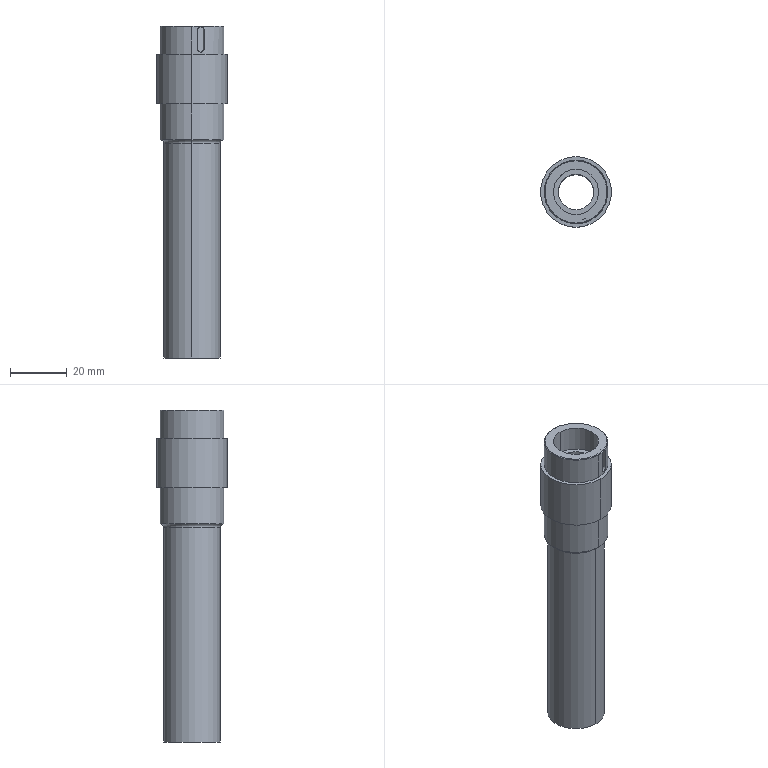Part | STEP file | 2026.6.15-Main Assembly图.sldasm-Part-95 | 1 solid | 26 faces | box 25 x 25 x 117.405 mm | volume 26751 mm3 | cylinder 14 | plane 8 | cone 2 | torus 2 | commonest cylinder face diameters 22.5 x4 2.5 x2 12.5 x2 16 x2 20 x2 25 x2
STEP:
#1=CARTESIAN_POINT('',(-1571.233,1430.514,3525.142));
#2=VERTEX_POINT('',#1);
#3=CARTESIAN_POINT('',(-1571.243,1418.014,3525.142));
#4=VERTEX_POINT('',#3);
#5=CARTESIAN_POINT('',(-1571.238,1424.264,3525.142));
#6=DIRECTION('',(0.,0.,1.));
#7=DIRECTION('',(1.,0.,0.));
#8=AXIS2_PLACEMENT_3D('',#5,#6,#7);
#9=CIRCLE('',#8,6.25);
#10=EDGE_CURVE('',#2,#4,#9,.T.);
#11=ORIENTED_EDGE('',*,*,#10,.F.);
#12=CARTESIAN_POINT('',(-1571.233,1430.514,3633.547));
#13=VERTEX_POINT('',#12);
#14=CARTESIAN_POINT('',(-1571.233,1430.514,3314.147));
#15=DIRECTION('',(0.,0.,1.));
#16=VECTOR('',#15,1000.);
#17=LINE('',#14,#16);
#18=EDGE_CURVE('',#2,#13,#17,.T.);
#19=ORIENTED_EDGE('',*,*,#18,.T.);
#20=CARTESIAN_POINT('',(-1571.243,1418.014,3633.547));
#21=VERTEX_POINT('',#20);
#22=CARTESIAN_POINT('',(-1571.238,1424.264,3633.547));
#23=DIRECTION('',(0.,0.,1.));
#24=DIRECTION('',(-0.0007664,-1.,0.));
#25=AXIS2_PLACEMENT_3D('',#22,#23,#24);
#26=CIRCLE('',#25,6.25);
#27=EDGE_CURVE('',#13,#21,#26,.T.);
#28=ORIENTED_EDGE('',*,*,#27,.T.);
#29=CARTESIAN_POINT('',(-1571.243,1418.014,3314.147));
#30=DIRECTION('',(0.,0.,1.));
#31=VECTOR('',#30,1000.);
#32=LINE('',#29,#31);
#33=EDGE_CURVE('',#4,#21,#32,.T.);
#34=ORIENTED_EDGE('',*,*,#33,.F.);
#35=EDGE_LOOP('',(#11,#19,#28,#34));
#36=FACE_OUTER_BOUND('',#35,.T.);
#37=CARTESIAN_POINT('',(-1571.238,1424.264,3314.147));
#38=DIRECTION('',(0.,0.,1.));
#39=DIRECTION('',(-0.0007664,-1.,0.));
#40=AXIS2_PLACEMENT_3D('',#37,#38,#39);
#41=CYLINDRICAL_SURFACE('',#40,6.25);
#42=ADVANCED_FACE('',(#36),#41,.F.);
#43=CARTESIAN_POINT('',(-1571.232,1432.264,3633.547));
#44=VERTEX_POINT('',#43);
#45=CARTESIAN_POINT('',(-1571.244,1416.264,3633.547));
#46=VERTEX_POINT('',#45);
#47=CARTESIAN_POINT('',(-1571.238,1424.264,3633.547));
#48=DIRECTION('',(0.,0.,1.));
#49=DIRECTION('',(-0.0007664,-1.,0.));
#50=AXIS2_PLACEMENT_3D('',#47,#48,#49);
#51=CIRCLE('',#50,8.);
#52=EDGE_CURVE('',#44,#46,#51,.T.);
#53=ORIENTED_EDGE('',*,*,#52,.F.);
#54=CARTESIAN_POINT('',(-1571.232,1432.264,3642.547));
#55=VERTEX_POINT('',#54);
#56=CARTESIAN_POINT('',(-1571.232,1432.264,3314.147));
#57=DIRECTION('',(0.,0.,1.));
#58=VECTOR('',#57,1000.);
#59=LINE('',#56,#58);
#60=EDGE_CURVE('',#44,#55,#59,.T.);
#61=ORIENTED_EDGE('',*,*,#60,.T.);
#62=CARTESIAN_POINT('',(-1571.244,1416.264,3642.547));
#63=VERTEX_POINT('',#62);
#64=CARTESIAN_POINT('',(-1571.238,1424.264,3642.547));
#65=DIRECTION('',(0.,0.,1.));
#66=DIRECTION('',(-0.0007664,-1.,0.));
#67=AXIS2_PLACEMENT_3D('',#64,#65,#66);
#68=CIRCLE('',#67,8.);
#69=EDGE_CURVE('',#55,#63,#68,.T.);
#70=ORIENTED_EDGE('',*,*,#69,.T.);
#71=CARTESIAN_POINT('',(-1571.244,1416.264,3314.147));
#72=DIRECTION('',(0.,0.,1.));
#73=VECTOR('',#72,1000.);
#74=LINE('',#71,#73);
#75=EDGE_CURVE('',#46,#63,#74,.T.);
#76=ORIENTED_EDGE('',*,*,#75,.F.);
#77=EDGE_LOOP('',(#53,#61,#70,#76));
#78=FACE_OUTER_BOUND('',#77,.T.);
#79=CARTESIAN_POINT('',(-1571.238,1424.264,3314.147));
#80=DIRECTION('',(0.,0.,1.));
#81=DIRECTION('',(-0.0007664,-1.,0.));
#82=AXIS2_PLACEMENT_3D('',#79,#80,#81);
#83=CYLINDRICAL_SURFACE('',#82,8.);
#84=ADVANCED_FACE('',(#78),#83,.F.);
#85=CARTESIAN_POINT('',(-1571.247,1413.264,3642.547));
#86=VERTEX_POINT('',#85);
#87=CARTESIAN_POINT('',(-1571.23,1435.264,3642.547));
#88=VERTEX_POINT('',#87);
#89=CARTESIAN_POINT('',(-1571.238,1424.264,3642.547));
#90=DIRECTION('',(0.,0.,1.));
#91=DIRECTION('',(-0.0007664,-1.,0.));
#92=AXIS2_PLACEMENT_3D('',#89,#90,#91);
#93=CIRCLE('',#92,11.);
#94=EDGE_CURVE('',#86,#88,#93,.T.);
#95=ORIENTED_EDGE('',*,*,#94,.F.);
#96=CARTESIAN_POINT('',(-1571.247,1413.014,3642.297));
#97=VERTEX_POINT('',#96);
#98=CARTESIAN_POINT('',(-1571.247,1413.264,3642.547));
#99=DIRECTION('',(-0.000542,-0.7071,-0.7071));
#100=VECTOR('',#99,1000.);
#101=LINE('',#98,#100);
#102=EDGE_CURVE('',#86,#97,#101,.T.);
#103=ORIENTED_EDGE('',*,*,#102,.T.);
#104=CARTESIAN_POINT('',(-1568.056,1413.474,3642.297));
#105=VERTEX_POINT('',#104);
#106=CARTESIAN_POINT('',(-1571.238,1424.264,3642.297));
#107=DIRECTION('',(0.,0.,1.));
#108=DIRECTION('',(-0.0007664,-1.,0.));
#109=AXIS2_PLACEMENT_3D('',#106,#107,#108);
#110=CIRCLE('',#109,11.25);
#111=EDGE_CURVE('',#97,#105,#110,.T.);
#112=ORIENTED_EDGE('',*,*,#111,.T.);
#113=CARTESIAN_POINT('',(-1571.23,1435.514,3642.297));
#114=VERTEX_POINT('',#113);
#115=CARTESIAN_POINT('',(-1571.238,1424.264,3642.297));
#116=DIRECTION('',(0.,0.,1.));
#117=DIRECTION('',(-0.0007664,-1.,0.));
#118=AXIS2_PLACEMENT_3D('',#115,#116,#117);
#119=CIRCLE('',#118,11.25);
#120=EDGE_CURVE('',#105,#114,#119,.T.);
#121=ORIENTED_EDGE('',*,*,#120,.T.);
#122=CARTESIAN_POINT('',(-1571.23,1435.264,3642.547));
#123=DIRECTION('',(0.000542,0.7071,-0.7071));
#124=VECTOR('',#123,1000.);
#125=LINE('',#122,#124);
#126=EDGE_CURVE('',#88,#114,#125,.T.);
#127=ORIENTED_EDGE('',*,*,#126,.F.);
#128=EDGE_LOOP('',(#95,#103,#112,#121,#127));
#129=FACE_OUTER_BOUND('',#128,.T.);
#130=CARTESIAN_POINT('',(-1571.238,1424.264,3642.547));
#131=DIRECTION('',(0.,0.,-1.));
#132=DIRECTION('',(0.0007664,1.,0.));
#133=AXIS2_PLACEMENT_3D('',#130,#131,#132);
#134=CONICAL_SURFACE('',#133,11.,0.7854);
#135=ADVANCED_FACE('',(#129),#134,.T.);
#136=CARTESIAN_POINT('',(-1571.247,1413.014,3632.547));
#137=VERTEX_POINT('',#136);
#138=CARTESIAN_POINT('',(-1571.23,1435.514,3632.547));
#139=VERTEX_POINT('',#138);
#140=CARTESIAN_POINT('',(-1571.238,1424.264,3632.547));
#141=DIRECTION('',(0.,0.,1.));
#142=DIRECTION('',(-0.0007664,-1.,0.));
#143=AXIS2_PLACEMENT_3D('',#140,#141,#142);
#144=CIRCLE('',#143,11.25);
#145=EDGE_CURVE('',#137,#139,#144,.T.);
#146=ORIENTED_EDGE('',*,*,#145,.T.);
#147=CARTESIAN_POINT('',(-1571.23,1435.514,3314.147));
#148=DIRECTION('',(0.,0.,1.));
#149=VECTOR('',#148,1000.);
#150=LINE('',#147,#149);
#151=EDGE_CURVE('',#139,#114,#150,.T.);
#152=ORIENTED_EDGE('',*,*,#151,.T.);
#153=ORIENTED_EDGE('',*,*,#120,.F.);
#154=CARTESIAN_POINT('',(-1566.877,1413.894,3641.047));
#155=VERTEX_POINT('',#154);
#156=CARTESIAN_POINT('',(-1566.877,1413.894,3641.047));
#157=CARTESIAN_POINT('',(-1566.877,1413.894,3641.212));
#158=CARTESIAN_POINT('',(-1566.907,1413.881,3641.374));
#159=CARTESIAN_POINT('',(-1567.024,1413.833,3641.677));
#160=CARTESIAN_POINT('',(-1567.11,1413.798,3641.816));
#161=CARTESIAN_POINT('',(-1567.326,1413.716,3642.046));
#162=CARTESIAN_POINT('',(-1567.458,1413.668,3642.139));
#163=CARTESIAN_POINT('',(-1567.743,1413.57,3642.264));
#164=CARTESIAN_POINT('',(-1567.899,1413.52,3642.297));
#165=CARTESIAN_POINT('',(-1568.056,1413.474,3642.297));
#166=B_SPLINE_CURVE_WITH_KNOTS('',3,(#156,#157,#158,#159,#160,#161,#162,#163,#164,#165),.UNSPECIFIED.,.F.,.F.,(4,2,2,2,4),(0.,0.000489,0.000978,0.001467,0.001956),.UNSPECIFIED.);
#167=EDGE_CURVE('',#155,#105,#166,.T.);
#168=ORIENTED_EDGE('',*,*,#167,.F.);
#169=CARTESIAN_POINT('',(-1566.877,1413.894,3634.547));
#170=VERTEX_POINT('',#169);
#171=CARTESIAN_POINT('',(-1566.877,1413.894,3314.147));
#172=DIRECTION('',(0.,0.,-1.));
#173=VECTOR('',#172,1000.);
#174=LINE('',#171,#173);
#175=EDGE_CURVE('',#155,#170,#174,.T.);
#176=ORIENTED_EDGE('',*,*,#175,.T.);
#177=CARTESIAN_POINT('',(-1569.275,1413.187,3634.547));
#178=VERTEX_POINT('',#177);
#179=CARTESIAN_POINT('',(-1569.275,1413.187,3634.547));
#180=CARTESIAN_POINT('',(-1569.275,1413.187,3634.382));
#181=CARTESIAN_POINT('',(-1569.242,1413.193,3634.219));
#182=CARTESIAN_POINT('',(-1569.118,1413.216,3633.917));
#183=CARTESIAN_POINT('',(-1569.027,1413.233,3633.778));
#184=CARTESIAN_POINT('',(-1568.801,1413.281,3633.548));
#185=CARTESIAN_POINT('',(-1568.664,1413.312,3633.455));
#186=CARTESIAN_POINT('',(-1568.372,1413.384,3633.33));
#187=CARTESIAN_POINT('',(-1568.213,1413.427,3633.297));
#188=CARTESIAN_POINT('',(-1567.979,1413.497,3633.297));
#189=CARTESIAN_POINT('',(-1567.899,1413.521,3633.305));
#190=CARTESIAN_POINT('',(-1567.747,1413.57,3633.337));
#191=CARTESIAN_POINT('',(-1567.673,1413.594,3633.36));
#192=CARTESIAN_POINT('',(-1567.457,1413.668,3633.454));
#193=CARTESIAN_POINT('',(-1567.328,1413.715,3633.546));
#194=CARTESIAN_POINT('',(-1567.109,1413.799,3633.779));
#195=CARTESIAN_POINT('',(-1567.024,1413.833,3633.916));
#196=CARTESIAN_POINT('',(-1566.907,1413.881,3634.219));
#197=CARTESIAN_POINT('',(-1566.877,1413.894,3634.382));
#198=CARTESIAN_POINT('',(-1566.877,1413.894,3634.547));
#199=B_SPLINE_CURVE_WITH_KNOTS('',3,(#179,#180,#181,#182,#183,#184,#185,#186,#187,#188,#189,#190,#191,#192,#193,#194,#195,#196,#197,#198),.UNSPECIFIED.,.F.,.F.,(4,2,2,2,2,2,2,2,2,4),(0.,0.0004888,0.0009776,0.001466,0.001955,0.002199,0.002444,0.002933,0.003421,0.00391),.UNSPECIFIED.);
#200=EDGE_CURVE('',#178,#170,#199,.T.);
#201=ORIENTED_EDGE('',*,*,#200,.F.);
#202=CARTESIAN_POINT('',(-1569.275,1413.187,3641.047));
#203=VERTEX_POINT('',#202);
#204=CARTESIAN_POINT('',(-1569.275,1413.187,3314.147));
#205=DIRECTION('',(0.,0.,1.));
#206=VECTOR('',#205,1000.);
#207=LINE('',#204,#206);
#208=EDGE_CURVE('',#178,#203,#207,.T.);
#209=ORIENTED_EDGE('',*,*,#208,.T.);
#210=CARTESIAN_POINT('',(-1568.056,1413.474,3642.297));
#211=CARTESIAN_POINT('',(-1568.134,1413.451,3642.297));
#212=CARTESIAN_POINT('',(-1568.214,1413.428,3642.289));
#213=CARTESIAN_POINT('',(-1568.369,1413.386,3642.257));
#214=CARTESIAN_POINT('',(-1568.444,1413.367,3642.233));
#215=CARTESIAN_POINT('',(-1568.665,1413.312,3642.139));
#216=CARTESIAN_POINT('',(-1568.799,1413.281,3642.048));
#217=CARTESIAN_POINT('',(-1569.028,1413.233,3641.814));
#218=CARTESIAN_POINT('',(-1569.118,1413.216,3641.677));
#219=CARTESIAN_POINT('',(-1569.242,1413.193,3641.375));
#220=CARTESIAN_POINT('',(-1569.275,1413.187,3641.212));
#221=CARTESIAN_POINT('',(-1569.275,1413.187,3641.047));
#222=B_SPLINE_CURVE_WITH_KNOTS('',3,(#210,#211,#212,#213,#214,#215,#216,#217,#218,#219,#220,#221),.UNSPECIFIED.,.F.,.F.,(4,2,2,2,2,4),(0.001956,0.0022,0.002445,0.002933,0.003422,0.00391),.UNSPECIFIED.);
#223=EDGE_CURVE('',#105,#203,#222,.T.);
#224=ORIENTED_EDGE('',*,*,#223,.F.);
#225=ORIENTED_EDGE('',*,*,#111,.F.);
#226=CARTESIAN_POINT('',(-1571.247,1413.014,3314.147));
#227=DIRECTION('',(0.,0.,1.));
#228=VECTOR('',#227,1000.);
#229=LINE('',#226,#228);
#230=EDGE_CURVE('',#137,#97,#229,.T.);
#231=ORIENTED_EDGE('',*,*,#230,.F.);
#232=EDGE_LOOP('',(#146,#152,#153,#168,#176,#201,#209,#224,#225,#231));
#233=FACE_OUTER_BOUND('',#232,.T.);
#234=CARTESIAN_POINT('',(-1571.238,1424.264,3314.147));
#235=DIRECTION('',(0.,0.,1.));
#236=DIRECTION('',(-0.0007664,-1.,0.));
#237=AXIS2_PLACEMENT_3D('',#234,#235,#236);
#238=CYLINDRICAL_SURFACE('',#237,11.25);
#239=ADVANCED_FACE('',(#233),#238,.T.);
#240=CARTESIAN_POINT('',(-1571.231,1434.264,3525.142));
#241=VERTEX_POINT('',#240);
#242=CARTESIAN_POINT('',(-1571.246,1414.264,3525.142));
#243=VERTEX_POINT('',#242);
#244=CARTESIAN_POINT('',(-1571.238,1424.264,3525.142));
#245=DIRECTION('',(0.,0.,-1.));
#246=DIRECTION('',(1.,0.,0.));
#247=AXIS2_PLACEMENT_3D('',#244,#245,#246);
#248=CIRCLE('',#247,10.);
#249=EDGE_CURVE('',#241,#243,#248,.T.);
#250=ORIENTED_EDGE('',*,*,#249,.F.);
#251=CARTESIAN_POINT('',(-1571.231,1434.264,3601.097));
#252=VERTEX_POINT('',#251);
#253=CARTESIAN_POINT('',(-1571.231,1434.264,3314.147));
#254=DIRECTION('',(0.,0.,1.));
#255=VECTOR('',#254,1000.);
#256=LINE('',#253,#255);
#257=EDGE_CURVE('',#241,#252,#256,.T.);
#258=ORIENTED_EDGE('',*,*,#257,.T.);
#259=CARTESIAN_POINT('',(-1571.246,1414.264,3601.097));
#260=VERTEX_POINT('',#259);
#261=CARTESIAN_POINT('',(-1571.238,1424.264,3601.097));
#262=DIRECTION('',(0.,0.,1.));
#263=DIRECTION('',(-0.0007664,-1.,0.));
#264=AXIS2_PLACEMENT_3D('',#261,#262,#263);
#265=CIRCLE('',#264,10.);
#266=EDGE_CURVE('',#260,#252,#265,.T.);
#267=ORIENTED_EDGE('',*,*,#266,.F.);
#268=CARTESIAN_POINT('',(-1571.246,1414.264,3314.147));
#269=DIRECTION('',(0.,0.,1.));
#270=VECTOR('',#269,1000.);
#271=LINE('',#268,#270);
#272=EDGE_CURVE('',#243,#260,#271,.T.);
#273=ORIENTED_EDGE('',*,*,#272,.F.);
#274=EDGE_LOOP('',(#250,#258,#267,#273));
#275=FACE_OUTER_BOUND('',#274,.T.);
#276=CARTESIAN_POINT('',(-1571.238,1424.264,3314.147));
#277=DIRECTION('',(0.,0.,1.));
#278=DIRECTION('',(-0.0007664,-1.,0.));
#279=AXIS2_PLACEMENT_3D('',#276,#277,#278);
#280=CYLINDRICAL_SURFACE('',#279,10.);
#281=ADVANCED_FACE('',(#275),#280,.T.);
#282=CARTESIAN_POINT('',(-1571.23,1435.514,3602.347));
#283=VERTEX_POINT('',#282);
#284=CARTESIAN_POINT('',(-1571.247,1413.014,3602.347));
#285=VERTEX_POINT('',#284);
#286=CARTESIAN_POINT('',(-1571.238,1424.264,3602.347));
#287=DIRECTION('',(0.,0.,1.));
#288=DIRECTION('',(-0.0007664,-1.,0.));
#289=AXIS2_PLACEMENT_3D('',#286,#287,#288);
#290=CIRCLE('',#289,11.25);
#291=EDGE_CURVE('',#283,#285,#290,.T.);
#292=ORIENTED_EDGE('',*,*,#291,.F.);
#293=CARTESIAN_POINT('',(-1571.23,1435.514,3601.097));
#294=DIRECTION('',(1.,-0.0007664,0.));
#295=DIRECTION('',(0.0007664,1.,0.));
#296=AXIS2_PLACEMENT_3D('',#293,#294,#295);
#297=CIRCLE('',#296,1.25);
#298=EDGE_CURVE('',#283,#252,#297,.T.);
#299=ORIENTED_EDGE('',*,*,#298,.T.);
#300=CARTESIAN_POINT('',(-1571.238,1424.264,3601.097));
#301=DIRECTION('',(0.,0.,1.));
#302=DIRECTION('',(-0.0007664,-1.,0.));
#303=AXIS2_PLACEMENT_3D('',#300,#301,#302);
#304=CIRCLE('',#303,10.);
#305=EDGE_CURVE('',#252,#260,#304,.T.);
#306=ORIENTED_EDGE('',*,*,#305,.T.);
#307=CARTESIAN_POINT('',(-1571.247,1413.014,3601.097));
#308=DIRECTION('',(-1.,0.0007664,0.));
#309=DIRECTION('',(-0.0007664,-1.,0.));
#310=AXIS2_PLACEMENT_3D('',#307,#308,#309);
#311=CIRCLE('',#310,1.25);
#312=EDGE_CURVE('',#285,#260,#311,.T.);
#313=ORIENTED_EDGE('',*,*,#312,.F.);
#314=EDGE_LOOP('',(#292,#299,#306,#313));
#315=FACE_OUTER_BOUND('',#314,.T.);
#316=CARTESIAN_POINT('',(-1571.238,1424.264,3601.097));
#317=DIRECTION('',(0.,0.,1.));
#318=DIRECTION('',(-0.0007664,-1.,0.));
#319=AXIS2_PLACEMENT_3D('',#316,#317,#318);
#320=TOROIDAL_SURFACE('',#319,11.25,1.25);
#321=ADVANCED_FACE('',(#315),#320,.F.);
#322=CARTESIAN_POINT('',(-1571.238,1424.264,3602.347));
#323=DIRECTION('',(0.,0.,1.));
#324=DIRECTION('',(-0.0007664,-1.,0.));
#325=AXIS2_PLACEMENT_3D('',#322,#323,#324);
#326=CIRCLE('',#325,11.25);
#327=EDGE_CURVE('',#285,#283,#326,.T.);
#328=ORIENTED_EDGE('',*,*,#327,.T.);
#329=CARTESIAN_POINT('',(-1571.23,1435.514,3615.047));
#330=VERTEX_POINT('',#329);
#331=CARTESIAN_POINT('',(-1571.23,1435.514,3314.147));
#332=DIRECTION('',(0.,0.,1.));
#333=VECTOR('',#332,1000.);
#334=LINE('',#331,#333);
#335=EDGE_CURVE('',#283,#330,#334,.T.);
#336=ORIENTED_EDGE('',*,*,#335,.T.);
#337=CARTESIAN_POINT('',(-1571.247,1413.014,3615.047));
#338=VERTEX_POINT('',#337);
#339=CARTESIAN_POINT('',(-1571.238,1424.264,3615.047));
#340=DIRECTION('',(0.,0.,1.));
#341=DIRECTION('',(-0.0007664,-1.,0.));
#342=AXIS2_PLACEMENT_3D('',#339,#340,#341);
#343=CIRCLE('',#342,11.25);
#344=EDGE_CURVE('',#338,#330,#343,.T.);
#345=ORIENTED_EDGE('',*,*,#344,.F.);
#346=CARTESIAN_POINT('',(-1571.247,1413.014,3314.147));
#347=DIRECTION('',(0.,0.,1.));
#348=VECTOR('',#347,1000.);
#349=LINE('',#346,#348);
#350=EDGE_CURVE('',#285,#338,#349,.T.);
#351=ORIENTED_EDGE('',*,*,#350,.F.);
#352=EDGE_LOOP('',(#328,#336,#345,#351));
#353=FACE_OUTER_BOUND('',#352,.T.);
#354=CARTESIAN_POINT('',(-1571.238,1424.264,3314.147));
#355=DIRECTION('',(0.,0.,1.));
#356=DIRECTION('',(-0.0007664,-1.,0.));
#357=AXIS2_PLACEMENT_3D('',#354,#355,#356);
#358=CYLINDRICAL_SURFACE('',#357,11.25);
#359=ADVANCED_FACE('',(#353),#358,.T.);
#360=CARTESIAN_POINT('',(-1571.248,1411.764,3615.047));
#361=VERTEX_POINT('',#360);
#362=CARTESIAN_POINT('',(-1571.229,1436.764,3615.047));
#363=VERTEX_POINT('',#362);
#364=CARTESIAN_POINT('',(-1571.238,1424.264,3615.047));
#365=DIRECTION('',(0.,0.,1.));
#366=DIRECTION('',(-0.0007664,-1.,0.));
#367=AXIS2_PLACEMENT_3D('',#364,#365,#366);
#368=CIRCLE('',#367,12.5);
#369=EDGE_CURVE('',#361,#363,#368,.T.);
#370=ORIENTED_EDGE('',*,*,#369,.T.);
#371=CARTESIAN_POINT('',(-1571.229,1436.764,3632.547));
#372=VERTEX_POINT('',#371);
#373=CARTESIAN_POINT('',(-1571.229,1436.764,3314.147));
#374=DIRECTION('',(0.,0.,1.));
#375=VECTOR('',#374,1000.);
#376=LINE('',#373,#375);
#377=EDGE_CURVE('',#363,#372,#376,.T.);
#378=ORIENTED_EDGE('',*,*,#377,.T.);
#379=CARTESIAN_POINT('',(-1571.248,1411.764,3632.547));
#380=VERTEX_POINT('',#379);
#381=CARTESIAN_POINT('',(-1571.238,1424.264,3632.547));
#382=DIRECTION('',(0.,0.,1.));
#383=DIRECTION('',(-0.0007664,-1.,0.));
#384=AXIS2_PLACEMENT_3D('',#381,#382,#383);
#385=CIRCLE('',#384,12.5);
#386=EDGE_CURVE('',#380,#372,#385,.T.);
#387=ORIENTED_EDGE('',*,*,#386,.F.);
#388=CARTESIAN_POINT('',(-1571.248,1411.764,3314.147));
#389=DIRECTION('',(0.,0.,1.));
#390=VECTOR('',#389,1000.);
#391=LINE('',#388,#390);
#392=EDGE_CURVE('',#361,#380,#391,.T.);
#393=ORIENTED_EDGE('',*,*,#392,.F.);
#394=EDGE_LOOP('',(#370,#378,#387,#393));
#395=FACE_OUTER_BOUND('',#394,.T.);
#396=CARTESIAN_POINT('',(-1571.238,1424.264,3314.147));
#397=DIRECTION('',(0.,0.,1.));
#398=DIRECTION('',(-0.0007664,-1.,0.));
#399=AXIS2_PLACEMENT_3D('',#396,#397,#398);
#400=CYLINDRICAL_SURFACE('',#399,12.5);
#401=ADVANCED_FACE('',(#395),#400,.T.);
#402=CARTESIAN_POINT('',(-1569.609,1414.319,3634.547));
#403=VERTEX_POINT('',#402);
#404=CARTESIAN_POINT('',(-1567.211,1415.026,3634.547));
#405=VERTEX_POINT('',#404);
#406=CARTESIAN_POINT('',(-1568.41,1414.673,3634.547));
#407=DIRECTION('',(0.2829,-0.9592,0.));
#408=DIRECTION('',(-0.9591,-0.2829,-0.004589));
#409=AXIS2_PLACEMENT_3D('',#406,#407,#408);
#410=CIRCLE('',#409,1.25);
#411=EDGE_CURVE('',#403,#405,#410,.T.);
#412=ORIENTED_EDGE('',*,*,#411,.T.);
#413=CARTESIAN_POINT('',(-1567.211,1415.026,3641.047));
#414=VERTEX_POINT('',#413);
#415=CARTESIAN_POINT('',(-1567.211,1415.026,3642.297));
#416=DIRECTION('',(0.,0.,1.));
#417=VECTOR('',#416,1000.);
#418=LINE('',#415,#417);
#419=EDGE_CURVE('',#405,#414,#418,.T.);
#420=ORIENTED_EDGE('',*,*,#419,.T.);
#421=CARTESIAN_POINT('',(-1569.609,1414.319,3641.047));
#422=VERTEX_POINT('',#421);
#423=CARTESIAN_POINT('',(-1568.41,1414.673,3641.047));
#424=DIRECTION('',(0.2829,-0.9592,0.));
#425=DIRECTION('',(-0.9591,-0.2829,-0.004589));
#426=AXIS2_PLACEMENT_3D('',#423,#424,#425);
#427=CIRCLE('',#426,1.25);
#428=EDGE_CURVE('',#414,#422,#427,.T.);
#429=ORIENTED_EDGE('',*,*,#428,.T.);
#430=CARTESIAN_POINT('',(-1569.609,1414.319,3642.297));
#431=DIRECTION('',(0.,0.,1.));
#432=VECTOR('',#431,1000.);
#433=LINE('',#430,#432);
#434=EDGE_CURVE('',#403,#422,#433,.T.);
#435=ORIENTED_EDGE('',*,*,#434,.F.);
#436=EDGE_LOOP('',(#412,#420,#429,#435));
#437=FACE_OUTER_BOUND('',#436,.T.);
#438=CARTESIAN_POINT('',(-1567.211,1415.026,3642.297));
#439=DIRECTION('',(-0.2829,0.9592,0.));
#440=DIRECTION('',(-0.9591,-0.2829,-0.004589));
#441=AXIS2_PLACEMENT_3D('',#438,#439,#440);
#442=PLANE('',#441);
#443=ADVANCED_FACE('',(#437),#442,.F.);
#444=CARTESIAN_POINT('',(-1569.609,1414.319,3634.547));
#445=DIRECTION('',(-0.2829,0.9592,0.));
#446=VECTOR('',#445,1000.);
#447=LINE('',#444,#446);
#448=EDGE_CURVE('',#178,#403,#447,.T.);
#449=ORIENTED_EDGE('',*,*,#448,.T.);
#450=ORIENTED_EDGE('',*,*,#434,.T.);
#451=CARTESIAN_POINT('',(-1569.609,1414.319,3641.047));
#452=DIRECTION('',(0.2829,-0.9592,0.));
#453=VECTOR('',#452,1000.);
#454=LINE('',#451,#453);
#455=EDGE_CURVE('',#422,#203,#454,.T.);
#456=ORIENTED_EDGE('',*,*,#455,.T.);
#457=ORIENTED_EDGE('',*,*,#208,.F.);
#458=EDGE_LOOP('',(#449,#450,#456,#457));
#459=FACE_OUTER_BOUND('',#458,.T.);
#460=CARTESIAN_POINT('',(-1569.609,1414.319,3642.297));
#461=DIRECTION('',(0.9592,0.2829,0.));
#462=DIRECTION('',(0.,0.,-1.));
#463=AXIS2_PLACEMENT_3D('',#460,#461,#462);
#464=PLANE('',#463);
#465=ADVANCED_FACE('',(#459),#464,.T.);
#466=ORIENTED_EDGE('',*,*,#200,.T.);
#467=CARTESIAN_POINT('',(-1567.211,1415.026,3634.547));
#468=DIRECTION('',(0.2829,-0.9592,0.));
#469=VECTOR('',#468,1000.);
#470=LINE('',#467,#469);
#471=EDGE_CURVE('',#405,#170,#470,.T.);
#472=ORIENTED_EDGE('',*,*,#471,.F.);
#473=ORIENTED_EDGE('',*,*,#411,.F.);
#474=ORIENTED_EDGE('',*,*,#448,.F.);
#475=EDGE_LOOP('',(#466,#472,#473,#474));
#476=FACE_OUTER_BOUND('',#475,.T.);
#477=CARTESIAN_POINT('',(-1568.41,1414.673,3634.547));
#478=DIRECTION('',(0.2829,-0.9592,0.));
#479=DIRECTION('',(0.9591,0.2829,0.004589));
#480=AXIS2_PLACEMENT_3D('',#477,#478,#479);
#481=CYLINDRICAL_SURFACE('',#480,1.25);
#482=ADVANCED_FACE('',(#476),#481,.F.);
#483=CARTESIAN_POINT('',(-1567.211,1415.026,3641.047));
#484=DIRECTION('',(-0.2829,0.9592,0.));
#485=VECTOR('',#484,1000.);
#486=LINE('',#483,#485);
#487=EDGE_CURVE('',#155,#414,#486,.T.);
#488=ORIENTED_EDGE('',*,*,#487,.T.);
#489=ORIENTED_EDGE('',*,*,#419,.F.);
#490=ORIENTED_EDGE('',*,*,#471,.T.);
#491=ORIENTED_EDGE('',*,*,#175,.F.);
#492=EDGE_LOOP('',(#488,#489,#490,#491));
#493=FACE_OUTER_BOUND('',#492,.T.);
#494=CARTESIAN_POINT('',(-1567.211,1415.026,3642.297));
#495=DIRECTION('',(0.9592,0.2829,0.));
#496=DIRECTION('',(0.,0.,-1.));
#497=AXIS2_PLACEMENT_3D('',#494,#495,#496);
#498=PLANE('',#497);
#499=ADVANCED_FACE('',(#493),#498,.F.);
#500=ORIENTED_EDGE('',*,*,#167,.T.);
#501=ORIENTED_EDGE('',*,*,#223,.T.);
#502=ORIENTED_EDGE('',*,*,#455,.F.);
#503=ORIENTED_EDGE('',*,*,#428,.F.);
#504=ORIENTED_EDGE('',*,*,#487,.F.);
#505=EDGE_LOOP('',(#500,#501,#502,#503,#504));
#506=FACE_OUTER_BOUND('',#505,.T.);
#507=CARTESIAN_POINT('',(-1568.41,1414.673,3641.047));
#508=DIRECTION('',(-0.2829,0.9592,0.));
#509=DIRECTION('',(-0.9591,-0.2829,-0.004589));
#510=AXIS2_PLACEMENT_3D('',#507,#508,#509);
#511=CYLINDRICAL_SURFACE('',#510,1.25);
#512=ADVANCED_FACE('',(#506),#511,.F.);
#513=ORIENTED_EDGE('',*,*,#386,.T.);
#514=CARTESIAN_POINT('',(-1571.238,1424.264,3632.547));
#515=DIRECTION('',(0.,0.,1.));
#516=DIRECTION('',(-0.0007664,-1.,0.));
#517=AXIS2_PLACEMENT_3D('',#514,#515,#516);
#518=CIRCLE('',#517,12.5);
#519=EDGE_CURVE('',#372,#380,#518,.T.);
#520=ORIENTED_EDGE('',*,*,#519,.T.);
#521=EDGE_LOOP('',(#513,#520));
#522=FACE_OUTER_BOUND('',#521,.T.);
#523=ORIENTED_EDGE('',*,*,#145,.F.);
#524=CARTESIAN_POINT('',(-1571.238,1424.264,3632.547));
#525=DIRECTION('',(0.,0.,1.));
#526=DIRECTION('',(-0.0007664,-1.,0.));
#527=AXIS2_PLACEMENT_3D('',#524,#525,#526);
#528=CIRCLE('',#527,11.25);
#529=EDGE_CURVE('',#139,#137,#528,.T.);
#530=ORIENTED_EDGE('',*,*,#529,.F.);
#531=EDGE_LOOP('',(#523,#530));
#532=FACE_BOUND('',#531,.T.);
#533=CARTESIAN_POINT('',(-1582.029,1421.082,3632.547));
#534=DIRECTION('',(0.,0.,1.));
#535=DIRECTION('',(-0.0007664,-1.,0.));
#536=AXIS2_PLACEMENT_3D('',#533,#534,#535);
#537=PLANE('',#536);
#538=ADVANCED_FACE('',(#522,#532),#537,.T.);
#539=ORIENTED_EDGE('',*,*,#377,.F.);
#540=CARTESIAN_POINT('',(-1571.238,1424.264,3615.047));
#541=DIRECTION('',(0.,0.,1.));
#542=DIRECTION('',(-0.0007664,-1.,0.));
#543=AXIS2_PLACEMENT_3D('',#540,#541,#542);
#544=CIRCLE('',#543,12.5);
#545=EDGE_CURVE('',#363,#361,#544,.T.);
#546=ORIENTED_EDGE('',*,*,#545,.T.);
#547=ORIENTED_EDGE('',*,*,#392,.T.);
#548=ORIENTED_EDGE('',*,*,#519,.F.);
#549=EDGE_LOOP('',(#539,#546,#547,#548));
#550=FACE_OUTER_BOUND('',#549,.T.);
#551=CARTESIAN_POINT('',(-1571.238,1424.264,3314.147));
#552=DIRECTION('',(0.,0.,1.));
#553=DIRECTION('',(-0.0007664,-1.,0.));
#554=AXIS2_PLACEMENT_3D('',#551,#552,#553);
#555=CYLINDRICAL_SURFACE('',#554,12.5);
#556=ADVANCED_FACE('',(#550),#555,.T.);
#557=ORIENTED_EDGE('',*,*,#344,.T.);
#558=CARTESIAN_POINT('',(-1571.238,1424.264,3615.047));
#559=DIRECTION('',(0.,0.,1.));
#560=DIRECTION('',(-0.0007664,-1.,0.));
#561=AXIS2_PLACEMENT_3D('',#558,#559,#560);
#562=CIRCLE('',#561,11.25);
#563=EDGE_CURVE('',#330,#338,#562,.T.);
#564=ORIENTED_EDGE('',*,*,#563,.T.);
#565=EDGE_LOOP('',(#557,#564));
#566=FACE_BOUND('',#565,.T.);
#567=ORIENTED_EDGE('',*,*,#369,.F.);
#568=ORIENTED_EDGE('',*,*,#545,.F.);
#569=EDGE_LOOP('',(#567,#568));
#570=FACE_OUTER_BOUND('',#569,.T.);
#571=CARTESIAN_POINT('',(-1583.228,1420.728,3615.047));
#572=DIRECTION('',(0.,0.,-1.));
#573=DIRECTION('',(0.0007664,1.,0.));
#574=AXIS2_PLACEMENT_3D('',#571,#572,#573);
#575=PLANE('',#574);
#576=ADVANCED_FACE('',(#566,#570),#575,.T.);
#577=ORIENTED_EDGE('',*,*,#335,.F.);
#578=ORIENTED_EDGE('',*,*,#291,.T.);
#579=ORIENTED_EDGE('',*,*,#350,.T.);
#580=ORIENTED_EDGE('',*,*,#563,.F.);
#581=EDGE_LOOP('',(#577,#578,#579,#580));
#582=FACE_OUTER_BOUND('',#581,.T.);
#583=CARTESIAN_POINT('',(-1571.238,1424.264,3314.147));
#584=DIRECTION('',(0.,0.,1.));
#585=DIRECTION('',(-0.0007664,-1.,0.));
#586=AXIS2_PLACEMENT_3D('',#583,#584,#585);
#587=CYLINDRICAL_SURFACE('',#586,11.25);
#588=ADVANCED_FACE('',(#582),#587,.T.);
#589=ORIENTED_EDGE('',*,*,#298,.F.);
#590=ORIENTED_EDGE('',*,*,#327,.F.);
#591=ORIENTED_EDGE('',*,*,#312,.T.);
#592=ORIENTED_EDGE('',*,*,#266,.T.);
#593=EDGE_LOOP('',(#589,#590,#591,#592));
#594=FACE_OUTER_BOUND('',#593,.T.);
#595=CARTESIAN_POINT('',(-1571.238,1424.264,3601.097));
#596=DIRECTION('',(0.,0.,1.));
#597=DIRECTION('',(-0.0007664,-1.,0.));
#598=AXIS2_PLACEMENT_3D('',#595,#596,#597);
#599=TOROIDAL_SURFACE('',#598,11.25,1.25);
#600=ADVANCED_FACE('',(#594),#599,.F.);
#601=ORIENTED_EDGE('',*,*,#257,.F.);
#602=CARTESIAN_POINT('',(-1571.238,1424.264,3525.142));
#603=DIRECTION('',(0.,0.,-1.));
#604=DIRECTION('',(1.,0.,0.));
#605=AXIS2_PLACEMENT_3D('',#602,#603,#604);
#606=CIRCLE('',#605,10.);
#607=EDGE_CURVE('',#243,#241,#606,.T.);
#608=ORIENTED_EDGE('',*,*,#607,.F.);
#609=ORIENTED_EDGE('',*,*,#272,.T.);
#610=ORIENTED_EDGE('',*,*,#305,.F.);
#611=EDGE_LOOP('',(#601,#608,#609,#610));
#612=FACE_OUTER_BOUND('',#611,.T.);
#613=CARTESIAN_POINT('',(-1571.238,1424.264,3314.147));
#614=DIRECTION('',(0.,0.,1.));
#615=DIRECTION('',(-0.0007664,-1.,0.));
#616=AXIS2_PLACEMENT_3D('',#613,#614,#615);
#617=CYLINDRICAL_SURFACE('',#616,10.);
#618=ADVANCED_FACE('',(#612),#617,.T.);
#619=ORIENTED_EDGE('',*,*,#151,.F.);
#620=ORIENTED_EDGE('',*,*,#529,.T.);
#621=ORIENTED_EDGE('',*,*,#230,.T.);
#622=CARTESIAN_POINT('',(-1571.238,1424.264,3642.297));
#623=DIRECTION('',(0.,0.,1.));
#624=DIRECTION('',(-0.0007664,-1.,0.));
#625=AXIS2_PLACEMENT_3D('',#622,#623,#624);
#626=CIRCLE('',#625,11.25);
#627=EDGE_CURVE('',#114,#97,#626,.T.);
#628=ORIENTED_EDGE('',*,*,#627,.F.);
#629=EDGE_LOOP('',(#619,#620,#621,#628));
#630=FACE_OUTER_BOUND('',#629,.T.);
#631=CARTESIAN_POINT('',(-1571.238,1424.264,3314.147));
#632=DIRECTION('',(0.,0.,1.));
#633=DIRECTION('',(-0.0007664,-1.,0.));
#634=AXIS2_PLACEMENT_3D('',#631,#632,#633);
#635=CYLINDRICAL_SURFACE('',#634,11.25);
#636=ADVANCED_FACE('',(#630),#635,.T.);
#637=ORIENTED_EDGE('',*,*,#102,.F.);
#638=CARTESIAN_POINT('',(-1571.238,1424.264,3642.547));
#639=DIRECTION('',(0.,0.,1.));
#640=DIRECTION('',(-0.0007664,-1.,0.));
#641=AXIS2_PLACEMENT_3D('',#638,#639,#640);
#642=CIRCLE('',#641,11.);
#643=EDGE_CURVE('',#88,#86,#642,.T.);
#644=ORIENTED_EDGE('',*,*,#643,.F.);
#645=ORIENTED_EDGE('',*,*,#126,.T.);
#646=ORIENTED_EDGE('',*,*,#627,.T.);
#647=EDGE_LOOP('',(#637,#644,#645,#646));
#648=FACE_OUTER_BOUND('',#647,.T.);
#649=CARTESIAN_POINT('',(-1571.238,1424.264,3642.547));
#650=DIRECTION('',(0.,0.,-1.));
#651=DIRECTION('',(0.0007664,1.,0.));
#652=AXIS2_PLACEMENT_3D('',#649,#650,#651);
#653=CONICAL_SURFACE('',#652,11.,0.7854);
#654=ADVANCED_FACE('',(#648),#653,.T.);
#655=ORIENTED_EDGE('',*,*,#643,.T.);
#656=ORIENTED_EDGE('',*,*,#94,.T.);
#657=EDGE_LOOP('',(#655,#656));
#658=FACE_OUTER_BOUND('',#657,.T.);
#659=CARTESIAN_POINT('',(-1571.238,1424.264,3642.547));
#660=DIRECTION('',(0.,0.,1.));
#661=DIRECTION('',(-0.0007664,-1.,0.));
#662=AXIS2_PLACEMENT_3D('',#659,#660,#661);
#663=CIRCLE('',#662,8.);
#664=EDGE_CURVE('',#63,#55,#663,.T.);
#665=ORIENTED_EDGE('',*,*,#664,.F.);
#666=ORIENTED_EDGE('',*,*,#69,.F.);
#667=EDGE_LOOP('',(#665,#666));
#668=FACE_BOUND('',#667,.T.);
#669=CARTESIAN_POINT('',(-1578.912,1422.001,3642.547));
#670=DIRECTION('',(0.,0.,1.));
#671=DIRECTION('',(-0.0007664,-1.,0.));
#672=AXIS2_PLACEMENT_3D('',#669,#670,#671);
#673=PLANE('',#672);
#674=ADVANCED_FACE('',(#658,#668),#673,.T.);
#675=ORIENTED_EDGE('',*,*,#60,.F.);
#676=CARTESIAN_POINT('',(-1571.238,1424.264,3633.547));
#677=DIRECTION('',(0.,0.,1.));
#678=DIRECTION('',(-0.0007664,-1.,0.));
#679=AXIS2_PLACEMENT_3D('',#676,#677,#678);
#680=CIRCLE('',#679,8.);
#681=EDGE_CURVE('',#46,#44,#680,.T.);
#682=ORIENTED_EDGE('',*,*,#681,.F.);
#683=ORIENTED_EDGE('',*,*,#75,.T.);
#684=ORIENTED_EDGE('',*,*,#664,.T.);
#685=EDGE_LOOP('',(#675,#682,#683,#684));
#686=FACE_OUTER_BOUND('',#685,.T.);
#687=CARTESIAN_POINT('',(-1571.238,1424.264,3314.147));
#688=DIRECTION('',(0.,0.,1.));
#689=DIRECTION('',(-0.0007664,-1.,0.));
#690=AXIS2_PLACEMENT_3D('',#687,#688,#689);
#691=CYLINDRICAL_SURFACE('',#690,8.);
#692=ADVANCED_FACE('',(#686),#691,.F.);
#693=ORIENTED_EDGE('',*,*,#681,.T.);
#694=ORIENTED_EDGE('',*,*,#52,.T.);
#695=EDGE_LOOP('',(#693,#694));
#696=FACE_OUTER_BOUND('',#695,.T.);
#697=CARTESIAN_POINT('',(-1571.238,1424.264,3633.547));
#698=DIRECTION('',(0.,0.,1.));
#699=DIRECTION('',(-0.0007664,-1.,0.));
#700=AXIS2_PLACEMENT_3D('',#697,#698,#699);
#701=CIRCLE('',#700,6.25);
#702=EDGE_CURVE('',#21,#13,#701,.T.);
#703=ORIENTED_EDGE('',*,*,#702,.F.);
#704=ORIENTED_EDGE('',*,*,#27,.F.);
#705=EDGE_LOOP('',(#703,#704));
#706=FACE_BOUND('',#705,.T.);
#707=CARTESIAN_POINT('',(-1577.233,1422.496,3633.547));
#708=DIRECTION('',(0.,0.,1.));
#709=DIRECTION('',(-0.0007664,-1.,0.));
#710=AXIS2_PLACEMENT_3D('',#707,#708,#709);
#711=PLANE('',#710);
#712=ADVANCED_FACE('',(#696,#706),#711,.T.);
#713=ORIENTED_EDGE('',*,*,#18,.F.);
#714=CARTESIAN_POINT('',(-1571.238,1424.264,3525.142));
#715=DIRECTION('',(0.,0.,1.));
#716=DIRECTION('',(1.,0.,0.));
#717=AXIS2_PLACEMENT_3D('',#714,#715,#716);
#718=CIRCLE('',#717,6.25);
#719=EDGE_CURVE('',#4,#2,#718,.T.);
#720=ORIENTED_EDGE('',*,*,#719,.F.);
#721=ORIENTED_EDGE('',*,*,#33,.T.);
#722=ORIENTED_EDGE('',*,*,#702,.T.);
#723=EDGE_LOOP('',(#713,#720,#721,#722));
#724=FACE_OUTER_BOUND('',#723,.T.);
#725=CARTESIAN_POINT('',(-1571.238,1424.264,3314.147));
#726=DIRECTION('',(0.,0.,1.));
#727=DIRECTION('',(-0.0007664,-1.,0.));
#728=AXIS2_PLACEMENT_3D('',#725,#726,#727);
#729=CYLINDRICAL_SURFACE('',#728,6.25);
#730=ADVANCED_FACE('',(#724),#729,.F.);
#731=ORIENTED_EDGE('',*,*,#607,.T.);
#732=ORIENTED_EDGE('',*,*,#249,.T.);
#733=EDGE_LOOP('',(#731,#732));
#734=FACE_OUTER_BOUND('',#733,.T.);
#735=ORIENTED_EDGE('',*,*,#719,.T.);
#736=ORIENTED_EDGE('',*,*,#10,.T.);
#737=EDGE_LOOP('',(#735,#736));
#738=FACE_BOUND('',#737,.T.);
#739=CARTESIAN_POINT('',(-1556.42,1410.832,3525.142));
#740=DIRECTION('',(0.,0.,1.));
#741=DIRECTION('',(1.,0.,0.));
#742=AXIS2_PLACEMENT_3D('',#739,#740,#741);
#743=PLANE('',#742);
#744=ADVANCED_FACE('',(#734,#738),#743,.F.);
#745=CLOSED_SHELL('',(#42,#84,#135,#239,#281,#321,#359,#401,#443,#465,#482,#499,#512,#538,#556,#576,#588,#600,#618,#636,#654,#674,#692,#712,#730,#744));
#746=MANIFOLD_SOLID_BREP('',#745);
#747=CARTESIAN_POINT('',(0.,0.,0.));
#748=DIRECTION('',(0.,0.,1.));
#749=DIRECTION('',(1.,0.,0.));
#750=AXIS2_PLACEMENT_3D('',#747,#748,#749);
#751=(LENGTH_UNIT()NAMED_UNIT(*)SI_UNIT(.MILLI.,.METRE.));
#752=UNCERTAINTY_MEASURE_WITH_UNIT(LENGTH_MEASURE(0.00001),#751,'','');
#753=(NAMED_UNIT(*)PLANE_ANGLE_UNIT()SI_UNIT($,.RADIAN.));
#754=(NAMED_UNIT(*)SI_UNIT($,.STERADIAN.)SOLID_ANGLE_UNIT());
#755=(GEOMETRIC_REPRESENTATION_CONTEXT(3)GLOBAL_UNCERTAINTY_ASSIGNED_CONTEXT((#752))GLOBAL_UNIT_ASSIGNED_CONTEXT((#751,#753,#754))REPRESENTATION_CONTEXT('',''));
#756=ADVANCED_BREP_SHAPE_REPRESENTATION('',(#746,#750),#755);